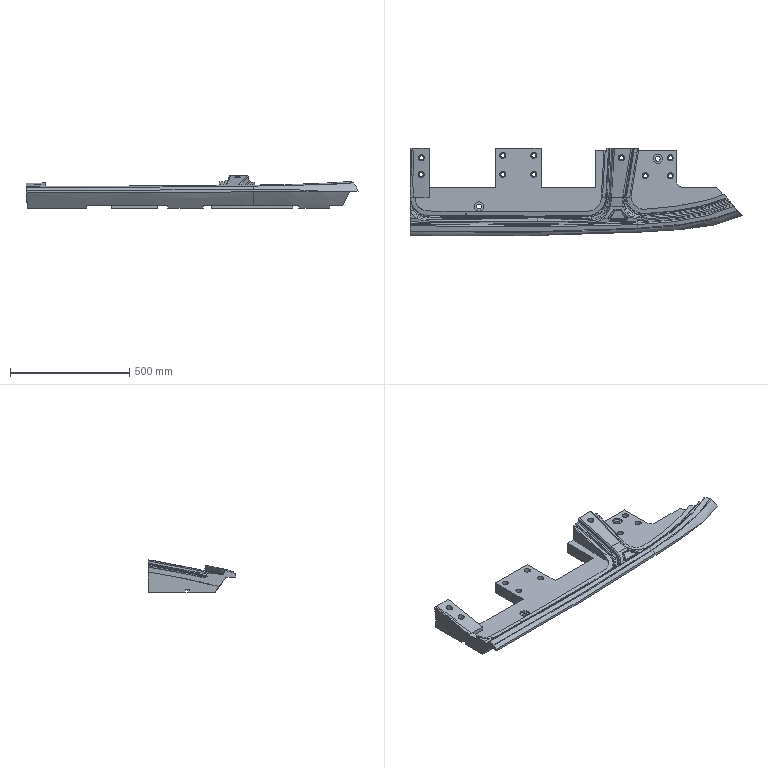Part | NX | features solid 2 | 1 solid | 258 faces | box 1394 x 368.502 x 135.762 mm | volume 16594186 mm3 | spline 173 | plane 60 | cylinder 25 | commonest cylinder face diameters 17 x10 25.5 x10 20 x2 40 x2 50 x1